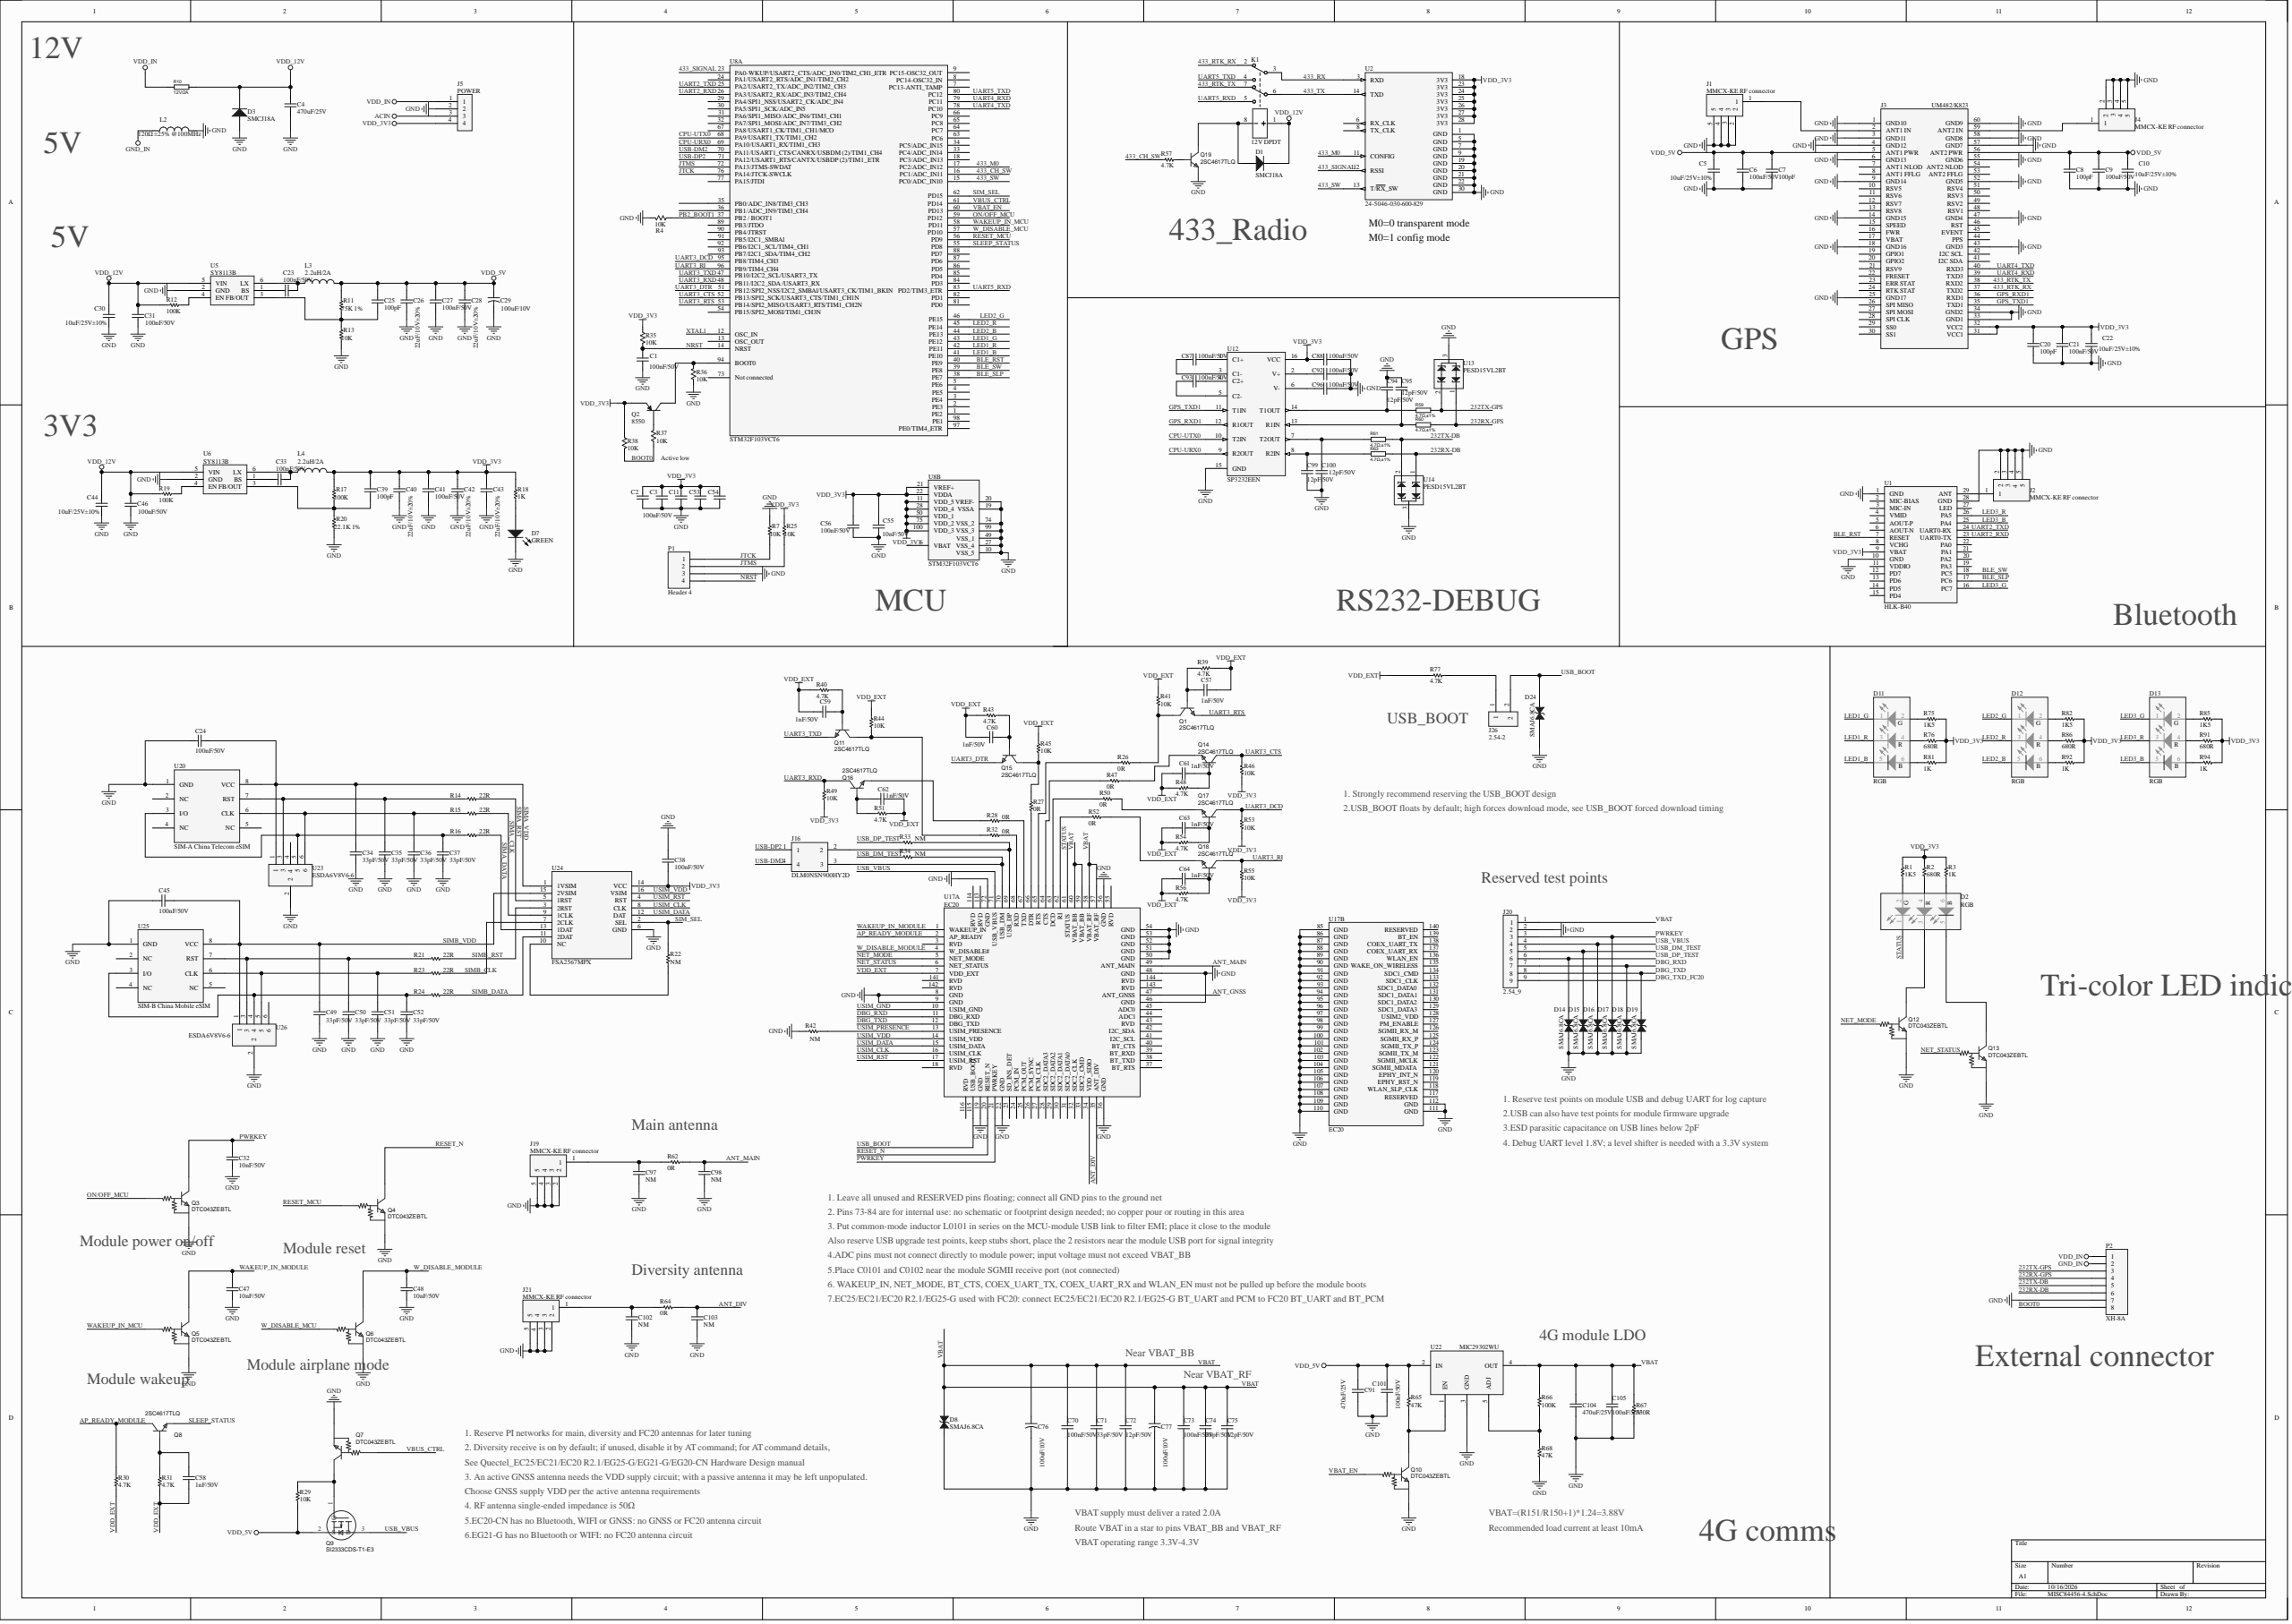Circuit board | Altium Designer | 219 parts | 170 nets
Bill of materials:
Comment,Description,Designator,Footprint,LibRef,Quantity
"100nF/50V","SMD capacitor, SMD ceramic capacitor, SMD capacitor,X7R","C1, C2, C3, C6, C9, C11, C21, C23, C24, C27, C31, C33, C38, C41, C45, C46, C53, C54, C56, C70, C73, C87, C88, C92, C93, C96, C101, C105","C0603","Cap","28"
"470uF/25V","470µF,25V,?8×11.5mm,RoHS","C4, C91, C104","RB8*11.5","Cap","3"
"10uF/25V±10%","SMD ceramic capacitor,X7R","C5, C10, C22, C30, C44","C1206","Cap","5"
"100pF","SMD ceramic capacitor","C7, C8, C20, C25, C39","C0603","Cap","5"
"22uF/10V±20%","SMD ceramic capacitor,X5R","C26, C28, C40, C42, C43","C0805","Cap","5"
"100uF/10V","100µF,10V,?5×7mm,RoHS","C29, C76, C77","RB5*7","Cap2","3"
"10nF/50V","SMD ceramic capacitor","C32, C47, C48","C0603","Cap","3"
"33pF/50V","SMD ceramic capacitor","C34, C35, C36, C37, C49, C50, C51, C52, C71, C74","C0603","Cap","10"
"10nF/50V","SMD capacitor","C55","C0805","Cap","1"
"1nF/50V","SMD ceramic capacitor","C57, C58, C59, C60, C61, C62, C63, C64","C0603","Cap","8"
"12pF/50V","SMD ceramic capacitor, SMD capacitor,X7R","C72, C75, C94, C95, C99, C100","C0603","Cap","6"
"NM","SMD ceramic capacitor","C97, C98, C102, C103","C0603","Cap","4"
"SMCJ18A","Default Diode","D1, D3","SMC","Diode","2"
"RGB","Full-color RGB LED,19-337C/RSBHGHC-M03/2T","D2, D11, D12, D13","RGB","LED1_3","4"
"GREEN","Typical RED GaAs LED","D7","LED0805","LED1","1"
"SMAJ6.8CA","SMD TVS diode","D8, D14, D15, D16, D17, D18, D19, D24","SMA","Diode_1","8"
"MMCX-KE RF connector","","J1, J2, J4, J19, J21","MMCX-KE","CIRCLE","5"
"UM482/K823","","J3","UM482/K823","UM482","1"
"POWER","","J5","2.54mm_2x2","2.54","1"
"DLM0NSN900HY2D","","J16","SMD_0.85x0.65mm","DLM0NSN900HY2D","1"
"2.54_9","","J20","2.54-9P","2.54_9","1"
"2.54-2","","J26","2.54mm-2P","2.54-2","1"
"12V DPDT","G6K-2P D12,OMRON","K1","G6K-2P D12","Relay-DPDT","1"
"120Ω ±25% @100MHz","Ferrite bead","L2","1812","Inductor","1"
"2.2uH/2A","SMD power inductor,cjiang(Changjiang Micro),FNR4026S2R2MT","L3, L4","SMD,4x4x2.6mm","Inductor","2"
"Header 4","Header, 4-Pin","P1","HDR1X4","Header 4","1"
"XH-8A","Header, 8-Pin","P2","XH-8A","Header 8","1"
"2SC4617TLQ","","Q1, Q8, Q11, Q14, Q15, Q16, Q17, Q18, Q19","SOT-416F_L1.6-W0.8-P1.00-LS1.6-TR","2SC4617TLQ","9"
"8550","PNP Bipolar Transistor","Q2","SOT-23","PNP","1"
"DTC043ZEBTL","","Q3, Q4, Q5, Q6, Q7, Q10, Q12, Q13","SOT-416_L1.6-W0.8-P1.00-LS1.6-BR","DTC043ZEBTL","8"
"SI2333CDS-T1-E3","","Q9","SOT-23_L2.9-W1.3-P1.90-LS2.4-BR","SI2333CDS-T1-E3","1"
"1K5","SMD resistor","R1, R75, R82, R85","R0603","Res1","4"
"680R","SMD resistor","R2, R76, R86, R91","R0603","Res1","4"
"1K","SMD resistor","R3, R18, R81, R92, R94","R0603","Res1","5"
"10K","SMD resistor , Resistor, SMD resistor","R4, R7, R13, R25, R29, R35, R36, R37, R38, R41, R44, R45, R46, R49, R53, R55","R0603","Res, Res1","16"
"12V/2A","Resettable fuse","R10","R1812","RES","1"
"75K 1%","Resistor","R11","R0603","Res1","1"
"100K","Resistor","R12, R17, R19, R66","R0603","Res1","4"
"22R","Resistor","R14, R15, R16, R21, R23, R24","R0603","Res1","6"
"22.1K 1%","Resistor","R20","R0603","Res1","1"
"NM","Resistor","R22, R33, R34, R42","R0603","Res1","4"
"0R","Resistor","R26, R27, R28, R32, R47, R50, R52, R62, R64","R0603","Res1","9"
"4.7K","Resistor","R30, R31, R39, R40, R43, R48, R51, R54, R56, R57, R77","R0603","Res1","11"
"4.7Ω,±1%","SMD resistor","R59, R60, R61, R63","R0603","RES","4"
"47K","Resistor","R65, R68","R0603","Res1","2"
"330R","Resistor","R67","R0603","Res1","1"
"HLK-B40","BLE5.1 Bluetooth module,Shenzhen Hi-Link","U1","HLK-B40","HLK-B40","1"
"24-5046-030-600-829","Kyocera Japan, 5046 series, mates HX-DU1006D","U2","HX-DU1006D","HX-DU1006D","1"
"SY8113B","","U5, U6","TSOT-23-6","SY8113B","2"
"STM32F103VCT6","Integrated IC","U8","LQFP-100_14x14x05P","STM32F103VBH6","1"
"SP3232EEN","","U12","SOP16-6.6","SP202ECT","1"
"PESD15VL2BT","","U13, U14","SOT-23","PESD12VL2BT","2"
"EC20","","U17","EC20","EC25/EC21","1"
"SIM-A China Telecom eSIM","","U20","VQFN8","SIM-A","1"
"MIC29302WU","","U22","TO-263-5","MIC29302WU","1"
"ESDA6V8V6-6","","U23, U26","SOT-563","ESDA6V8V6-6","2"
"FSA2567MPX","","U24","MLP-16","FSA2567","1"
"SIM-B China Mobile eSIM","","U25","DFN2*2-8","SIM-A","1"
Netlist (Protel format):
[
C1
C0603
100nF/50V



]
[
C2
C0603
100nF/50V



]
[
C3
C0603
100nF/50V



]
[
C4
RB8*11.5
470uF/25V



]
[
C5
C1206
10uF/25V±10%



]
[
C6
C0603
100nF/50V



]
[
C7
C0603
100pF



]
[
C8
C0603
100pF



]
[
C9
C0603
100nF/50V



]
[
C10
C1206
10uF/25V±10%



]
[
C11
C0603
100nF/50V



]
[
C20
C0603
100pF



]
[
C21
C0603
100nF/50V



]
[
C22
C1206
10uF/25V±10%



]
[
C23
C0603
100nF/50V



]
[
C24
C0603
100nF/50V



]
[
C25
C0603
100pF



]
[
C26
C0805
22uF/10V±20%



]
[
C27
C0603
100nF/50V



]
[
C28
C0805
22uF/10V±20%



]
[
C29
RB5*7
100uF/10V



]
[
C30
C1206
10uF/25V±10%



]
[
C31
C0603
100nF/50V



]
[
C32
C0603
10nF/50V



]
[
C33
C0603
100nF/50V



]
[
C34
C0603
33pF/50V



]
[
C35
C0603
33pF/50V



]
[
C36
C0603
33pF/50V



]
[
C37
C0603
33pF/50V



]
[
C38
C0603
100nF/50V



]
[
C39
C0603
100pF



]
[
C40
C0805
22uF/10V±20%



]
[
C41
C0603
100nF/50V



]
[
C42
C0805
22uF/10V±20%



]
[
C43
C0805
22uF/10V±20%



]
[
C44
C1206
10uF/25V±10%



]
[
C45
C0603
100nF/50V



]
[
C46
C0603
100nF/50V



]
[
C47
C0603
10nF/50V



]
[
C48
C0603
10nF/50V



]
[
C49
C0603
33pF/50V



]
[
C50
C0603
33pF/50V



]
[
C51
C0603
33pF/50V



]
[
C52
C0603
33pF/50V



]
[
C53
C0603
100nF/50V



]
[
C54
C0603
100nF/50V



]
[
C55
C0805
10nF/50V



]
[
C56
C0603
100nF/50V



]
[
C57
C0603
1nF/50V



]
[
C58
C0603
1nF/50V



]
[
C59
C0603
1nF/50V



]
[
C60
C0603
1nF/50V



]
[
C61
C0603
1nF/50V



]
[
C62
C0603
1nF/50V



]
[
C63
C0603
1nF/50V



]
[
C64
C0603
1nF/50V



]
[
C70
C0603
100nF/50V



]
[
C71
C0603
33pF/50V



]
[
C72
C0603
12pF/50V



]
[
C73
C0603
100nF/50V



]
[
C74
C0603
33pF/50V



]
[
C75
C0603
12pF/50V



]
[
C76
RB5*7
100uF/10V



]
[
C77
RB5*7
100uF/10V



]
[
C87
C0603
100nF/50V



]
[
C88
C0603
100nF/50V



]
[
C91
RB8*11.5
470uF/25V



]
[
C92
C0603
100nF/50V



]
[
C93
C0603
100nF/50V



]
[
C94
C0603
12pF/50V



]
[
C95
C0603
12pF/50V



]
[
C96
C0603
100nF/50V



]
[
C97
C0603
NM



]
[
C98
C0603
NM



]
[
C99
C0603
12pF/50V



]
[
C100
C0603
12pF/50V



]
[
C101
C0603
100nF/50V



]
[
C102
C0603
NM



]
[
C103
C0603
NM



]
[
C104
RB8*11.5
470uF/25V



]
[
C105
C0603
100nF/50V



]
[
D1
SMC
SMCJ18A



]
[
D2
RGB
RGB



]
[
D3
SMC
SMCJ18A



]
[
D7
LED0805
GREEN



]
[
D8
SMA
SMAJ6.8CA



]
[
D11
RGB
RGB



]
[
D12
RGB
RGB



]
[
D13
RGB
RGB



]
[
D14
SMA
SMAJ6.8CA



]
[
D15
SMA
SMAJ6.8CA



]
[
D16
SMA
SMAJ6.8CA



]
[
D17
SMA
SMAJ6.8CA



]
[
D18
SMA
SMAJ6.8CA



]
[
D19
SMA
SMAJ6.8CA



]
[
D24
SMA
SMAJ6.8CA



]
[
J1
MMCX-KE
MMCX-KE RF connector



]
[
J2
MMCX-KE
MMCX-KE RF connector



]
[
J3
UM482/K823
UM482/K823



]
[
J4
MMCX-KE
MMCX-KE RF connector



]
[
J5
2.54mm_2x2
POWER



]
[
J16
SMD_0.85x0.65mm
DLM0NSN900HY2D



]
[
J19
MMCX-KE
MMCX-KE RF connector



]
[
J20
2.54-9P
2.54_9



]
[
J21
MMCX-KE
MMCX-KE RF connector



]
[
J26
2.54mm-2P
2.54-2



]
[
K1
G6K-2P D12
12V DPDT



]
[
L2
1812
120Ω ±25% @100MHz



]
[
L3
SMD,4x4x2.6mm
2.2uH/2A



]
[
L4
SMD,4x4x2.6mm
2.2uH/2A



]
[
P1
HDR1X4
Header 4



]
[
P2
XH-8A
XH-8A



]
[
Q1
SOT-416F_L1.6-W0.8-P1.00-LS1.6-TR
2SC4617TLQ



]
[
Q2
SOT-23
8550



]
[
Q3
SOT-416_L1.6-W0.8-P1.00-LS1.6-BR
DTC043ZEBTL



]
[
Q4
SOT-416_L1.6-W0.8-P1.00-LS1.6-BR
DTC043ZEBTL



]
[
Q5
SOT-416_L1.6-W0.8-P1.00-LS1.6-BR
DTC043ZEBTL



]
[
Q6
SOT-416_L1.6-W0.8-P1.00-LS1.6-BR
DTC043ZEBTL



]
[
Q7
SOT-416_L1.6-W0.8-P1.00-LS1.6-BR
DTC043ZEBTL



]
[
Q8
SOT-416F_L1.6-W0.8-P1.00-LS1.6-TR
2SC4617TLQ



]
[
Q9
SOT-23_L2.9-W1.3-P1.90-LS2.4-BR
SI2333CDS-T1-E3



]
[
Q10
SOT-416_L1.6-W0.8-P1.00-LS1.6-BR
DTC043ZEBTL



]
[
Q11
SOT-416F_L1.6-W0.8-P1.00-LS1.6-TR
2SC4617TLQ



]
[
Q12
SOT-416_L1.6-W0.8-P1.00-LS1.6-BR
DTC043ZEBTL



]
[
Q13
SOT-416_L1.6-W0.8-P1.00-LS1.6-BR
DTC043ZEBTL



]
[
Q14
SOT-416F_L1.6-W0.8-P1.00-LS1.6-TR
2SC4617TLQ



]
[
Q15
SOT-416F_L1.6-W0.8-P1.00-LS1.6-TR
2SC4617TLQ



]
[
Q16
SOT-416F_L1.6-W0.8-P1.00-LS1.6-TR
2SC4617TLQ



]
[
Q17
SOT-416F_L1.6-W0.8-P1.00-LS1.6-TR
2SC4617TLQ



]
[
Q18
SOT-416F_L1.6-W0.8-P1.00-LS1.6-TR
2SC4617TLQ



]
[
Q19
SOT-416F_L1.6-W0.8-P1.00-LS1.6-TR
2SC4617TLQ



]
[
R1
R0603
1K5



]
[
R2
R0603
680R



]
[
R3
R0603
1K



]
[
R4
R0603
10K



]
[
R7
R0603
10K



]
[
R10
R1812
12V/2A



]
[
R11
R0603
75K 1%



]
[
R12
R0603
100K



]
[
R13
R0603
10K



]
[
R14
R0603
22R



]
[
R15
R0603
22R



]
[
R16
R0603
22R



]
[
R17
R0603
100K



]
[
R18
R0603
1K



]
[
R19
R0603
100K



]
[
R20
R0603
22.1K 1%



]
[
R21
R0603
22R



]
[
R22
R0603
NM



]
[
R23
R0603
22R



]
[
R24
R0603
22R



]
[
R25
R0603
10K



]
[
R26
R0603
0R



]
[
R27
R0603
0R



]
[
R28
R0603
0R



]
[
R29
R0603
10K



]
[
R30
R0603
4.7K



]
[
R31
R0603
4.7K



]
[
R32
R0603
0R



]
[
R33
R0603
NM



]
[
R34
R0603
NM



]
[
R35
R0603
10K



]
[
R36
R0603
10K



]
[
R37
R0603
10K



]
[
R38
R0603
10K



]
[
R39
R0603
4.7K



]
[
R40
R0603
4.7K



]
[
R41
R0603
10K



]
[
R42
R0603
NM



]
[
R43
R0603
4.7K



]
[
R44
R0603
10K



]
[
R45
R0603
10K



]
[
R46
R0603
10K



]
[
R47
R0603
0R



]
[
R48
R0603
4.7K



]
[
R49
R0603
10K



]
[
R50
R0603
0R



]
[
R51
R0603
4.7K



]
[
R52
R0603
0R



]
[
R53
R0603
10K



]
[
R54
R0603
4.7K



]
[
R55
R0603
10K



]
[
R56
R0603
4.7K



]
[
R57
R0603
4.7K



]
[
R59
R0603
4.7Ω,±1%



]
[
R60
R0603
4.7Ω,±1%



]
[
R61
R0603
4.7Ω,±1%



]
[
R62
R0603
0R



]
[
R63
R0603
4.7Ω,±1%



]
[
R64
R0603
0R



]
[
R65
R0603
47K



]
[
R66
R0603
100K



]
[
R67
R0603
330R



]
[
R68
R0603
47K



]
[
R75
R0603
1K5



]
[
R76
R0603
680R



]
[
R77
R0603
4.7K



]
[
R81
R0603
1K



]
[
R82
R0603
1K5



]
[
R85
R0603
1K5



]
[
R86
R0603
680R



]
[
R91
R0603
680R



]
[
R92
R0603
1K



]
[
R94
R0603
1K



]
[
U1
HLK-B40
HLK-B40



]
[
U2
HX-DU1006D
24-5046-030-600-829



]
[
U5
TSOT-23-6
SY8113B



]
[
U6
TSOT-23-6
SY8113B



]
[
U8
LQFP-100_14x14x05P
STM32F103VCT6



]
[
U12
SOP16-6.6
SP3232EEN



]
[
U13
SOT-23
PESD15VL2BT



]
[
U14
SOT-23
PESD15VL2BT



]
[
U17
EC20
EC20



]
[
U20
VQFN8
SIM-A China Telecom eSIM



]
[
U22
TO-263-5
MIC29302WU



]
[
U23
SOT-563
ESDA6V8V6-6



]
[
U24
MLP-16
FSA2567MPX



]
[
U25
DFN2*2-8
SIM-B China Mobile eSIM



]
[
U26
SOT-563
ESDA6V8V6-6



]
(
WAKEUP_IN_MODULE
C47-1
Q5-3
U17-1
)
(
WAKEUP_IN_MCU
Q5-1
U8-58
)
(
W_DISABLE_MODULE
C48-1
Q6-3
U17-4
)
(
W_DISABLE_MCU
Q6-1
U8-57
)
(
VDD_IN
J5-1
P2-1
R10-2
)
(
VDD_EXT
C57-1
C58-2
C59-1
C60-1
C61-2
C62-2
C63-2
C64-2
R30-1
R31-1
R39-2
R40-2
R41-1
R43-2
R44-1
R45-1
R48-1
R51-1
R54-1
R56-1
R77-1
U17-7
)
(
VDD_12V
C4-1
C30-2
C31-2
C44-2
C46-2
D1-2
D3-2
K1-1
R10-1
R12-2
R19-2
U5-5
U6-5
)
(
VDD_5V
C5-2
C6-1
C7-1
C8-2
C9-2
C10-2
C25-1
C26-1
C27-1
C28-1
C29-1
C91-1
C101-1
J3-5
J3-56
L3-2
Q9-2
R11-2
R29-1
R65-2
U22-2
)
(
VDD_3V3
C2-1
C3-1
C11-1
C20-2
C21-2
C22-2
C38-2
C39-1
C40-1
C41-1
C42-1
C43-1
C53-1
C54-1
C55-2
C56-1
C88-1
J3-31
J3-32
J5-4
L4-2
Q2-2
R1-1
R2-1
R3-1
R17-2
R18-1
R25-2
R35-2
R38-2
R46-2
R49-2
R53-2
R55-2
R75-1
R76-1
R81-1
R82-1
R85-1
R86-1
R91-1
R92-1
R94-1
U1-9
U2-18
U2-23
U2-24
U2-25
U2-26
U2-27
U2-28
U8-11
U8-21
U8-22
U8-28
U8-50
U8-75
U8-100
U12-16
U24-14
)
(
VBUS_CTRL
Q7-1
U8-61
)
(
VBAT_EN
Q10-1
U8-60
)
(
VBAT
C70-1
C71-1
C72-1
C73-1
C74-1
C75-1
C76-1
C77-1
C104-1
C105-1
D8-2
J20-1
R66-2
R67-2
U17-57
U17-58
U17-59
U17-60
U22-4
)
(
USIM_VDD
U17-14
U24-16
)
(
USIM_RST
U17-17
U24-4
)
(
USIM_PRESENCE
R42-2
U17-13
)
(
USIM_DATA
U17-15
U24-12
)
(
USIM_CLK
U17-16
U24-8
)
(
USB_VBUS
D16-2
J20-4
Q9-3
U17-71
)
(
USB_DP_TEST
D14-2
J20-6
R33-1
)
(
USB_DM_TEST
D15-2
J20-5
R34-1
)
(
USB_BOOT
D24-2
J26-2
U17-115
)
(
USB-DP2
J16-1
U8-71
)
(
USB-DM2
J16-4
U8-70
)
(
UART5_TXD
K1-4
U8-80
)
(
UART5_RXD
K1-5
U8-83
)
(
UART4_TXD
J3-40
U8-78
)
(
UART4_RXD
J3-39
U8-79
)
(
UART3_TXD
Q11-1
U8-47
)
(
UART3_RXD
Q16-3
R49-1
U8-48
)
(
UART3_RTS
Q1-1
U8-53
)
(
UART3_RI
Q18-3
R55-1
U8-96
)
(
UART3_DTR
Q15-1
U8-51
)
(
UART3_DCD
Q17-3
R53-1
U8-95
)
(
UART3_CTS
Q14-3
R46-1
U8-52
)
(
UART2_TXD
U1-24
U8-25
)
(
UART2_RXD
U1-23
U8-26
)
(
STATUS
D2-1
U17-61
)
(
SLEEP_STATUS
Q8-1
U8-55
)
(
SIMB_VDD
C45-1
C49-1
U24-15
U25-8
U26-1
)
(
SIMB_RST
R21-1
U24-3
)
(
SIMB_DATA
R24-1
U24-11
)
(
SIMB_CLK
R23-1
U24-7
)
(
SIMA_VDD
C24-1
C34-1
U20-8
U23-1
U24-1
)
(
SIMA_RST
R14-1
U24-5
)
(
SIMA_DATA
R16-1
U24-13
)
(
SIMA_CLK
R15-1
U24-9
)
(
SIM_SEL
R22-1
U8-62
U24-2
)
(
RESET_N
Q4-3
U17-20
)
(
RESET_MCU
Q4-1
U8-56
)
(
PWRKEY
C32-1
D17-2
J20-3
Q3-3
U17-21
)
(
PB2_BOOT1
R4-2
U8-37
)
(
ON/OFF_MCU
Q3-1
U8-59
)
(
NRST
C1-2
P1-4
R35-1
U8-14
)
(
NetR66_1
R66-1
R68-2
U22-5
)
(
NetR52_2
R52-2
U17-62
)
(
NetR50_2
R50-2
U17-63
)
(
NetR47_2
R47-2
U17-64
)
(
NetR32_2
R32-2
U17-68
)
(
NetR28_2
R28-2
U17-67
)
(
NetR27_2
R27-2
U17-66
)
(
NetR26_2
R26-2
U17-65
)
(
NetR22_2
R22-2
U24-10
)
(
NetR19_1
R19-1
U6-4
)
(
NetR12_1
R12-1
U5-4
)
(
NetQ19_2
Q19-2
R57-1
)
(
NetQ18_1
Q18-1
R52-1
)
(
NetQ17_1
Q17-1
R50-1
)
(
NetQ16_1
Q16-1
R28-1
)
(
NetQ15_3
Q15-3
R27-1
R45-2
)
(
NetQ14_1
Q14-1
R47-1
)
(
NetQ11_3
Q11-3
R32-1
R44-2
)
(
NetQ10_3
Q10-3
R65-1
U22-1
)
(
NetQ7_3
Q7-3
Q9-1
R29-2
)
(
NetQ2_3
Q2-3
R36-2
U8-94
)
(
NetQ2_1
Q2-1
R37-1
)
(
NetQ1_3
Q1-3
R26-1
R41-2
)
(
NetJ26_1
J26-1
R77-2
)
(
NetJ16_3
J16-3
R34-2
U17-70
)
(
NetJ16_2
J16-2
R33-2
U17-69
)
(
NetJ3_59
J3-59
J4-1
)
(
NetJ2_1
J2-1
U1-29
)
(
NetJ1_1
J1-1
J3-2
)
(
NetD13_6
D13-6
R94-2
)
(
NetD13_4
D13-4
R91-2
)
(
NetD13_2
D13-2
R85-2
)
(
NetD12_6
D12-6
R92-2
)
(
NetD12_4
D12-4
R86-2
)
(
NetD12_2
D12-2
R82-2
)
(
NetD11_6
D11-6
R81-2
)
(
NetD11_4
D11-4
R76-2
)
(
NetD11_2
D11-2
R75-2
)
(
NetD7_1
D7-1
R18-2
)
(
NetD2_6
D2-6
R3-2
)
(
NetD2_5
D2-5
Q13-3
)
(
NetD2_4
D2-4
R2-2
)
(
NetD2_3
D2-3
Q12-3
)
(
NetD2_2
D2-2
R1-2
)
(
NetD1_1
D1-1
K1-8
Q19-3
)
(
NetC102_2
C102-2
J21-1
R64-2
)
(
NetC100_1
C100-1
R61-2
U12-7
)
(
NetC99_1
C99-1
R63-2
U12-8
)
(
NetC97_2
C97-2
J19-1
R62-2
)
(
NetC96_1
C96-1
U12-6
)
(
NetC95_2
C95-2
R60-2
U12-13
)
(
NetC94_2
C94-2
R59-2
U12-14
)
(
NetC93_2
C93-2
U12-4
)
(
NetC93_1
C93-1
U12-5
)
(
NetC92_1
C92-1
U12-2
)
(
NetC87_2
C87-2
U12-1
)
(
NetC87_1
C87-1
U12-3
)
(
NetC64_1
C64-1
Q18-2
R56-2
)
(
NetC63_1
C63-1
Q17-2
R54-2
)
(
NetC62_1
C62-1
Q16-2
R51-2
)
(
NetC61_1
C61-1
Q14-2
R48-2
)
(
NetC60_2
C60-2
Q15-2
R43-1
)
(
NetC59_2
C59-2
Q11-2
R40-1
)
(
NetC58_1
C58-1
Q8-2
R31-2
)
(
NetC57_2
C57-2
Q1-2
R39-1
)
(
NetC52_1
C52-1
R24-2
U25-3
U26-4
)
(
NetC51_1
C51-1
R23-2
U25-6
U26-5
)
(
NetC50_1
C50-1
R21-2
U25-7
U26-3
)
(
NetC39_2
C39-2
R17-1
R20-2
U6-3
)
(
NetC37_1
C37-1
R16-2
U20-3
U23-5
)
(
NetC36_1
C36-1
R15-2
U20-6
U23-6
)
(
NetC35_1
C35-1
R14-2
U20-7
U23-3
)
(
NetC33_2
C33-2
U6-1
)
(
NetC33_1
C33-1
L4-1
U6-6
)
(
NetC25_2
C25-2
R11-1
R13-2
U5-3
)
(
NetC23_2
C23-2
U5-1
)
(
NetC23_1
C23-1
L3-1
U5-6
)
(
NET_STATUS
Q13-1
U17-6
)
(
NET_MODE
Q12-1
U17-5
)
(
LED3_R
D13-3
U1-26
)
(
LED3_G
D13-1
U1-16
)
(
LED3_B
D13-5
U1-25
)
(
LED2_R
D12-3
U8-45
)
(
LED2_G
D12-1
U8-46
)
(
LED2_B
D12-5
U8-44
)
(
LED1_R
D11-3
U8-42
)
(
LED1_G
D11-1
U8-43
)
(
LED1_B
D11-5
U8-41
)
(
JTMS
P1-2
R25-1
U8-72
)
(
JTCK
P1-1
R7-1
U8-76
)
(
GPS_TXD1
J3-35
U12-11
)
(
GPS_RXD1
J3-36
U12-12
)
(
GND_IN
L2-1
P2-2
)
(
GND
C1-1
C2-2
C3-2
C4-2
C5-1
C6-2
C7-2
C8-1
C9-1
C10-1
C11-2
C20-1
C21-1
C22-1
C24-2
C26-2
C27-2
C28-2
C29-2
C30-1
C31-1
C32-2
C34-2
C35-2
C36-2
C37-2
C38-1
C40-2
C41-2
C42-2
C43-2
C44-1
C45-2
C46-1
C47-2
C48-2
C49-2
C50-2
C51-2
C52-2
C53-2
C54-2
C55-1
C56-2
C70-2
C71-2
C72-2
C73-2
C74-2
C75-2
C76-2
C77-2
C88-2
C91-2
C92-2
C94-1
C95-1
C96-2
C97-1
C98-1
C99-2
C100-2
C101-2
C102-1
C103-1
C104-2
C105-2
D3-1
D7-2
D8-1
D14-1
D15-1
D16-1
D17-1
D18-1
D19-1
D24-1
J1-2
J1-3
J1-4
J1-5
J2-2
J2-3
J2-4
J2-5
J3-1
J3-3
J3-4
J3-6
J3-9
J3-14
J3-18
J3-25
J3-33
J3-34
J3-43
J3-47
J3-52
J3-55
J3-57
J3-58
J3-60
J4-2
J4-3
J4-4
J4-5
J5-2
J19-2
J19-3
J19-4
J19-5
J20-2
J21-2
J21-3
J21-4
J21-5
L2-2
P1-3
P2-7
Q3-2
Q4-2
Q5-2
Q6-2
Q7-2
Q10-2
Q12-2
Q13-2
Q19-1
R4-1
R7-2
R13-1
R20-1
R36-1
R42-1
R67-1
R68-1
U1-1
U1-10
U1-28
U2-1
U2-5
U2-7
U2-9
U2-19
U2-20
U2-21
U2-22
U2-30
U5-2
U6-2
U8-10
U8-19
U8-20
U8-27
U8-49
U8-74
U8-99
U12-15
U13-3
U14-3
U17-8
U17-9
U17-19
U17-22
U17-36
U17-46
U17-48
U17-50
U17-51
U17-52
U17-53
U17-54
U17-56
U17-72
U17-85
U17-86
U17-87
U17-88
U17-89
U17-90
U17-91
U17-92
U17-93
U17-94
U17-95
U17-96
U17-97
U17-98
U17-99
U17-100
U17-101
U17-102
U17-103
U17-104
U17-105
U17-106
U17-107
U17-108
U17-109
U17-110
U17-111
U17-112
U20-1
U22-3
U23-2
U24-6
U25-1
U26-2
)
(
DBG_TXD
D19-2
J20-8
U17-12
)
(
DBG_RXD
D18-2
J20-7
U17-11
)
(
CPU-UTX0
U8-68
U12-10
)
(
CPU-URX0
U8-69
U12-9
)
(
BOOT0
P2-8
R37-2
R38-1
)
(
BLE_SW
U1-18
U8-39
)
(
BLE_SLP
U1-17
U8-38
)
(
BLE_RST
U1-7
U8-40
)
(
AP_READY_MODULE
Q8-3
R30-2
U17-2
)
(
ANT_MAIN
C98-2
R62-1
U17-49
)
(
ANT_DIV
C103-2
R64-1
U17-35
)
(
433_TX
K1-6
U2-14
)
(
433_SW
U2-13
U8-15
)
(
433_SIGNAL
U2-12
U8-23
)
(
433_RX
K1-3
U2-3
)
(
433_RTK_TX
J3-38
K1-7
)
(
433_RTK_RX
J3-37
K1-2
)
(
433_M0
U2-11
U8-17
)
(
433_CH_SW
R57-2
U8-16
)
(
232TX-GPS
P2-3
R59-1
U13-2
)
(
232TX-DB
P2-5
R61-1
U14-2
)
(
232RX-GPS
P2-4
R60-1
U13-1
)
(
232RX-DB
P2-6
R63-1
U14-1
)